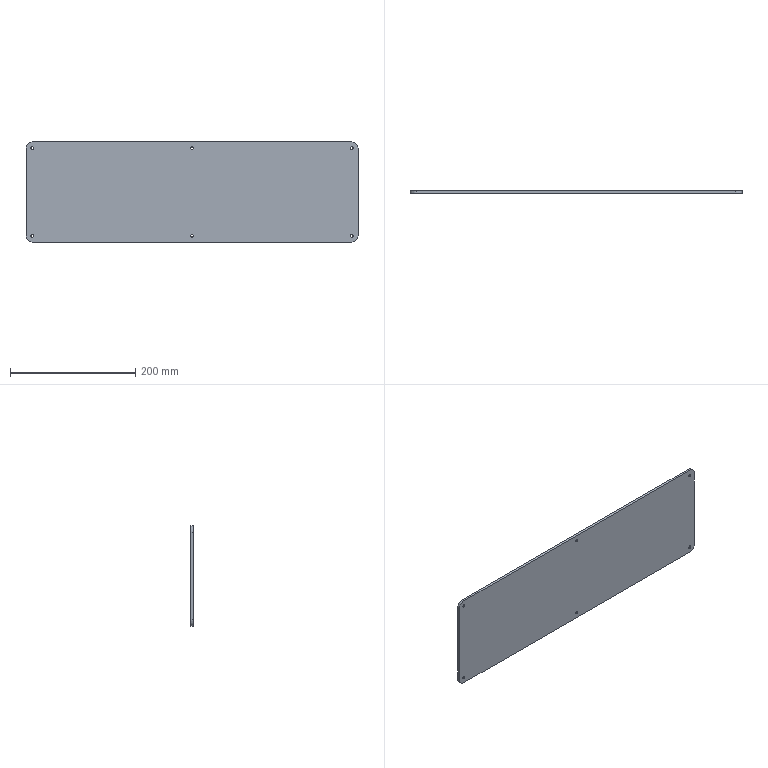Part | NX | 1 solid | 22 faces | box 530 x 4 x 160 mm | volume 338194 mm3 | cylinder 10 | plane 6 | cone 6 | commonest cylinder face diameters 4.5 x6 20 x4
STEP:
#1=CARTESIAN_POINT('',(265.,4.,70.));
#2=VERTEX_POINT('',#1);
#3=CARTESIAN_POINT('',(265.,4.,-70.));
#4=VERTEX_POINT('',#3);
#5=CARTESIAN_POINT('',(265.,4.,-80.));
#6=DIRECTION('',(0.,0.,-1.));
#7=VECTOR('',#6,1000.);
#8=LINE('',#5,#7);
#9=EDGE_CURVE('',#2,#4,#8,.T.);
#10=ORIENTED_EDGE('',*,*,#9,.F.);
#11=CARTESIAN_POINT('',(265.,0.,70.));
#12=VERTEX_POINT('',#11);
#13=CARTESIAN_POINT('',(265.,4.,70.));
#14=DIRECTION('',(0.,-1.,0.));
#15=VECTOR('',#14,1000.);
#16=LINE('',#13,#15);
#17=EDGE_CURVE('',#2,#12,#16,.T.);
#18=ORIENTED_EDGE('',*,*,#17,.T.);
#19=CARTESIAN_POINT('',(265.,0.,-70.));
#20=VERTEX_POINT('',#19);
#21=CARTESIAN_POINT('',(265.,0.,-80.));
#22=DIRECTION('',(0.,0.,-1.));
#23=VECTOR('',#22,1000.);
#24=LINE('',#21,#23);
#25=EDGE_CURVE('',#12,#20,#24,.T.);
#26=ORIENTED_EDGE('',*,*,#25,.T.);
#27=CARTESIAN_POINT('',(265.,4.,-70.));
#28=DIRECTION('',(0.,-1.,0.));
#29=VECTOR('',#28,1000.);
#30=LINE('',#27,#29);
#31=EDGE_CURVE('',#20,#4,#30,.F.);
#32=ORIENTED_EDGE('',*,*,#31,.T.);
#33=EDGE_LOOP('',(#10,#18,#26,#32));
#34=FACE_BOUND('',#33,.T.);
#35=CARTESIAN_POINT('',(265.,4.,-80.));
#36=DIRECTION('',(-1.,0.,0.));
#37=DIRECTION('',(0.,0.,1.));
#38=AXIS2_PLACEMENT_3D('',#35,#36,#37);
#39=PLANE('',#38);
#40=ADVANCED_FACE('',(#34),#39,.F.);
#41=CARTESIAN_POINT('',(255.,4.,-80.));
#42=VERTEX_POINT('',#41);
#43=CARTESIAN_POINT('',(-255.,4.,-80.));
#44=VERTEX_POINT('',#43);
#45=CARTESIAN_POINT('',(-265.,4.,-80.));
#46=DIRECTION('',(-1.,0.,0.));
#47=VECTOR('',#46,1000.);
#48=LINE('',#45,#47);
#49=EDGE_CURVE('',#42,#44,#48,.T.);
#50=ORIENTED_EDGE('',*,*,#49,.F.);
#51=CARTESIAN_POINT('',(255.,0.,-80.));
#52=VERTEX_POINT('',#51);
#53=CARTESIAN_POINT('',(255.,4.,-80.));
#54=DIRECTION('',(0.,-1.,0.));
#55=VECTOR('',#54,1000.);
#56=LINE('',#53,#55);
#57=EDGE_CURVE('',#42,#52,#56,.T.);
#58=ORIENTED_EDGE('',*,*,#57,.T.);
#59=CARTESIAN_POINT('',(-255.,0.,-80.));
#60=VERTEX_POINT('',#59);
#61=CARTESIAN_POINT('',(-265.,0.,-80.));
#62=DIRECTION('',(-1.,0.,0.));
#63=VECTOR('',#62,1000.);
#64=LINE('',#61,#63);
#65=EDGE_CURVE('',#52,#60,#64,.T.);
#66=ORIENTED_EDGE('',*,*,#65,.T.);
#67=CARTESIAN_POINT('',(-255.,4.,-80.));
#68=DIRECTION('',(0.,-1.,0.));
#69=VECTOR('',#68,1000.);
#70=LINE('',#67,#69);
#71=EDGE_CURVE('',#60,#44,#70,.F.);
#72=ORIENTED_EDGE('',*,*,#71,.T.);
#73=EDGE_LOOP('',(#50,#58,#66,#72));
#74=FACE_BOUND('',#73,.T.);
#75=CARTESIAN_POINT('',(-265.,4.,-80.));
#76=DIRECTION('',(0.,0.,1.));
#77=DIRECTION('',(1.,0.,0.));
#78=AXIS2_PLACEMENT_3D('',#75,#76,#77);
#79=PLANE('',#78);
#80=ADVANCED_FACE('',(#74),#79,.F.);
#81=CARTESIAN_POINT('',(-265.,0.,-70.));
#82=VERTEX_POINT('',#81);
#83=CARTESIAN_POINT('',(-265.,0.,70.));
#84=VERTEX_POINT('',#83);
#85=CARTESIAN_POINT('',(-265.,0.,-80.));
#86=DIRECTION('',(0.,0.,1.));
#87=VECTOR('',#86,1000.);
#88=LINE('',#85,#87);
#89=EDGE_CURVE('',#82,#84,#88,.T.);
#90=ORIENTED_EDGE('',*,*,#89,.T.);
#91=CARTESIAN_POINT('',(-265.,4.,70.));
#92=VERTEX_POINT('',#91);
#93=CARTESIAN_POINT('',(-265.,4.,70.));
#94=DIRECTION('',(0.,-1.,0.));
#95=VECTOR('',#94,1000.);
#96=LINE('',#93,#95);
#97=EDGE_CURVE('',#84,#92,#96,.F.);
#98=ORIENTED_EDGE('',*,*,#97,.T.);
#99=CARTESIAN_POINT('',(-265.,4.,-70.));
#100=VERTEX_POINT('',#99);
#101=CARTESIAN_POINT('',(-265.,4.,-80.));
#102=DIRECTION('',(0.,0.,1.));
#103=VECTOR('',#102,1000.);
#104=LINE('',#101,#103);
#105=EDGE_CURVE('',#100,#92,#104,.T.);
#106=ORIENTED_EDGE('',*,*,#105,.F.);
#107=CARTESIAN_POINT('',(-265.,4.,-70.));
#108=DIRECTION('',(0.,-1.,0.));
#109=VECTOR('',#108,1000.);
#110=LINE('',#107,#109);
#111=EDGE_CURVE('',#100,#82,#110,.T.);
#112=ORIENTED_EDGE('',*,*,#111,.T.);
#113=EDGE_LOOP('',(#90,#98,#106,#112));
#114=FACE_BOUND('',#113,.T.);
#115=CARTESIAN_POINT('',(-265.,4.,-80.));
#116=DIRECTION('',(1.,0.,0.));
#117=DIRECTION('',(0.,0.,-1.));
#118=AXIS2_PLACEMENT_3D('',#115,#116,#117);
#119=PLANE('',#118);
#120=ADVANCED_FACE('',(#114),#119,.F.);
#121=CARTESIAN_POINT('',(-255.,0.,80.));
#122=VERTEX_POINT('',#121);
#123=CARTESIAN_POINT('',(255.,0.,80.));
#124=VERTEX_POINT('',#123);
#125=CARTESIAN_POINT('',(-265.,0.,80.));
#126=DIRECTION('',(1.,0.,0.));
#127=VECTOR('',#126,1000.);
#128=LINE('',#125,#127);
#129=EDGE_CURVE('',#122,#124,#128,.T.);
#130=ORIENTED_EDGE('',*,*,#129,.T.);
#131=CARTESIAN_POINT('',(255.,4.,80.));
#132=VERTEX_POINT('',#131);
#133=CARTESIAN_POINT('',(255.,4.,80.));
#134=DIRECTION('',(0.,-1.,0.));
#135=VECTOR('',#134,1000.);
#136=LINE('',#133,#135);
#137=EDGE_CURVE('',#124,#132,#136,.F.);
#138=ORIENTED_EDGE('',*,*,#137,.T.);
#139=CARTESIAN_POINT('',(-255.,4.,80.));
#140=VERTEX_POINT('',#139);
#141=CARTESIAN_POINT('',(-265.,4.,80.));
#142=DIRECTION('',(1.,0.,0.));
#143=VECTOR('',#142,1000.);
#144=LINE('',#141,#143);
#145=EDGE_CURVE('',#140,#132,#144,.T.);
#146=ORIENTED_EDGE('',*,*,#145,.F.);
#147=CARTESIAN_POINT('',(-255.,4.,80.));
#148=DIRECTION('',(0.,-1.,0.));
#149=VECTOR('',#148,1000.);
#150=LINE('',#147,#149);
#151=EDGE_CURVE('',#140,#122,#150,.T.);
#152=ORIENTED_EDGE('',*,*,#151,.T.);
#153=EDGE_LOOP('',(#130,#138,#146,#152));
#154=FACE_BOUND('',#153,.T.);
#155=CARTESIAN_POINT('',(-265.,4.,80.));
#156=DIRECTION('',(0.,0.,-1.));
#157=DIRECTION('',(-1.,0.,0.));
#158=AXIS2_PLACEMENT_3D('',#155,#156,#157);
#159=PLANE('',#158);
#160=ADVANCED_FACE('',(#154),#159,.F.);
#161=CARTESIAN_POINT('',(-255.,4.,74.48));
#162=VERTEX_POINT('',#161);
#163=CARTESIAN_POINT('',(-255.,4.,70.));
#164=DIRECTION('',(0.,1.,0.));
#165=DIRECTION('',(0.,0.,1.));
#166=AXIS2_PLACEMENT_3D('',#163,#164,#165);
#167=CIRCLE('',#166,4.48);
#168=EDGE_CURVE('',#162,#162,#167,.T.);
#169=ORIENTED_EDGE('',*,*,#168,.F.);
#170=EDGE_LOOP('',(#169));
#171=FACE_BOUND('',#170,.T.);
#172=CARTESIAN_POINT('',(-255.,4.,-65.52));
#173=VERTEX_POINT('',#172);
#174=CARTESIAN_POINT('',(-255.,4.,-70.));
#175=DIRECTION('',(0.,1.,0.));
#176=DIRECTION('',(0.,0.,1.));
#177=AXIS2_PLACEMENT_3D('',#174,#175,#176);
#178=CIRCLE('',#177,4.48);
#179=EDGE_CURVE('',#173,#173,#178,.T.);
#180=ORIENTED_EDGE('',*,*,#179,.F.);
#181=EDGE_LOOP('',(#180));
#182=FACE_BOUND('',#181,.T.);
#183=CARTESIAN_POINT('',(255.,4.,74.48));
#184=VERTEX_POINT('',#183);
#185=CARTESIAN_POINT('',(255.,4.,70.));
#186=DIRECTION('',(0.,1.,0.));
#187=DIRECTION('',(0.,0.,1.));
#188=AXIS2_PLACEMENT_3D('',#185,#186,#187);
#189=CIRCLE('',#188,4.48);
#190=EDGE_CURVE('',#184,#184,#189,.T.);
#191=ORIENTED_EDGE('',*,*,#190,.F.);
#192=EDGE_LOOP('',(#191));
#193=FACE_BOUND('',#192,.T.);
#194=CARTESIAN_POINT('',(255.,4.,-65.52));
#195=VERTEX_POINT('',#194);
#196=CARTESIAN_POINT('',(255.,4.,-70.));
#197=DIRECTION('',(0.,1.,0.));
#198=DIRECTION('',(0.,0.,1.));
#199=AXIS2_PLACEMENT_3D('',#196,#197,#198);
#200=CIRCLE('',#199,4.48);
#201=EDGE_CURVE('',#195,#195,#200,.T.);
#202=ORIENTED_EDGE('',*,*,#201,.F.);
#203=EDGE_LOOP('',(#202));
#204=FACE_BOUND('',#203,.T.);
#205=CARTESIAN_POINT('',(0.,4.,-65.52));
#206=VERTEX_POINT('',#205);
#207=CARTESIAN_POINT('',(0.,4.,-70.));
#208=DIRECTION('',(0.,1.,0.));
#209=DIRECTION('',(0.,0.,1.));
#210=AXIS2_PLACEMENT_3D('',#207,#208,#209);
#211=CIRCLE('',#210,4.48);
#212=EDGE_CURVE('',#206,#206,#211,.T.);
#213=ORIENTED_EDGE('',*,*,#212,.F.);
#214=EDGE_LOOP('',(#213));
#215=FACE_BOUND('',#214,.T.);
#216=CARTESIAN_POINT('',(0.,4.,74.48));
#217=VERTEX_POINT('',#216);
#218=CARTESIAN_POINT('',(0.,4.,70.));
#219=DIRECTION('',(0.,1.,0.));
#220=DIRECTION('',(0.,0.,1.));
#221=AXIS2_PLACEMENT_3D('',#218,#219,#220);
#222=CIRCLE('',#221,4.48);
#223=EDGE_CURVE('',#217,#217,#222,.T.);
#224=ORIENTED_EDGE('',*,*,#223,.F.);
#225=EDGE_LOOP('',(#224));
#226=FACE_BOUND('',#225,.T.);
#227=ORIENTED_EDGE('',*,*,#145,.T.);
#228=CARTESIAN_POINT('',(255.,4.,70.));
#229=DIRECTION('',(0.,1.,0.));
#230=DIRECTION('',(0.,0.,1.));
#231=AXIS2_PLACEMENT_3D('',#228,#229,#230);
#232=CIRCLE('',#231,10.);
#233=EDGE_CURVE('',#132,#2,#232,.T.);
#234=ORIENTED_EDGE('',*,*,#233,.T.);
#235=ORIENTED_EDGE('',*,*,#9,.T.);
#236=CARTESIAN_POINT('',(255.,4.,-70.));
#237=DIRECTION('',(0.,1.,0.));
#238=DIRECTION('',(0.,0.,1.));
#239=AXIS2_PLACEMENT_3D('',#236,#237,#238);
#240=CIRCLE('',#239,10.);
#241=EDGE_CURVE('',#4,#42,#240,.T.);
#242=ORIENTED_EDGE('',*,*,#241,.T.);
#243=ORIENTED_EDGE('',*,*,#49,.T.);
#244=CARTESIAN_POINT('',(-255.,4.,-70.));
#245=DIRECTION('',(0.,1.,0.));
#246=DIRECTION('',(0.,0.,1.));
#247=AXIS2_PLACEMENT_3D('',#244,#245,#246);
#248=CIRCLE('',#247,10.);
#249=EDGE_CURVE('',#44,#100,#248,.T.);
#250=ORIENTED_EDGE('',*,*,#249,.T.);
#251=ORIENTED_EDGE('',*,*,#105,.T.);
#252=CARTESIAN_POINT('',(-255.,4.,70.));
#253=DIRECTION('',(0.,1.,0.));
#254=DIRECTION('',(0.,0.,1.));
#255=AXIS2_PLACEMENT_3D('',#252,#253,#254);
#256=CIRCLE('',#255,10.);
#257=EDGE_CURVE('',#92,#140,#256,.T.);
#258=ORIENTED_EDGE('',*,*,#257,.T.);
#259=EDGE_LOOP('',(#227,#234,#235,#242,#243,#250,#251,#258));
#260=FACE_BOUND('',#259,.T.);
#261=CARTESIAN_POINT('',(0.,4.,0.));
#262=DIRECTION('',(0.,1.,0.));
#263=DIRECTION('',(0.,0.,1.));
#264=AXIS2_PLACEMENT_3D('',#261,#262,#263);
#265=PLANE('',#264);
#266=ADVANCED_FACE('',(#171,#182,#193,#204,#215,#226,#260),#265,.T.);
#267=CARTESIAN_POINT('',(-255.,0.,72.25));
#268=VERTEX_POINT('',#267);
#269=CARTESIAN_POINT('',(-255.,0.,70.));
#270=DIRECTION('',(0.,1.,0.));
#271=DIRECTION('',(0.,0.,1.));
#272=AXIS2_PLACEMENT_3D('',#269,#270,#271);
#273=CIRCLE('',#272,2.25);
#274=EDGE_CURVE('',#268,#268,#273,.T.);
#275=ORIENTED_EDGE('',*,*,#274,.T.);
#276=EDGE_LOOP('',(#275));
#277=FACE_BOUND('',#276,.T.);
#278=CARTESIAN_POINT('',(-255.,0.,-67.75));
#279=VERTEX_POINT('',#278);
#280=CARTESIAN_POINT('',(-255.,0.,-70.));
#281=DIRECTION('',(0.,1.,0.));
#282=DIRECTION('',(0.,0.,1.));
#283=AXIS2_PLACEMENT_3D('',#280,#281,#282);
#284=CIRCLE('',#283,2.25);
#285=EDGE_CURVE('',#279,#279,#284,.T.);
#286=ORIENTED_EDGE('',*,*,#285,.T.);
#287=EDGE_LOOP('',(#286));
#288=FACE_BOUND('',#287,.T.);
#289=CARTESIAN_POINT('',(255.,0.,72.25));
#290=VERTEX_POINT('',#289);
#291=CARTESIAN_POINT('',(255.,0.,70.));
#292=DIRECTION('',(0.,1.,0.));
#293=DIRECTION('',(0.,0.,1.));
#294=AXIS2_PLACEMENT_3D('',#291,#292,#293);
#295=CIRCLE('',#294,2.25);
#296=EDGE_CURVE('',#290,#290,#295,.T.);
#297=ORIENTED_EDGE('',*,*,#296,.T.);
#298=EDGE_LOOP('',(#297));
#299=FACE_BOUND('',#298,.T.);
#300=CARTESIAN_POINT('',(255.,0.,-67.75));
#301=VERTEX_POINT('',#300);
#302=CARTESIAN_POINT('',(255.,0.,-70.));
#303=DIRECTION('',(0.,1.,0.));
#304=DIRECTION('',(0.,0.,1.));
#305=AXIS2_PLACEMENT_3D('',#302,#303,#304);
#306=CIRCLE('',#305,2.25);
#307=EDGE_CURVE('',#301,#301,#306,.T.);
#308=ORIENTED_EDGE('',*,*,#307,.T.);
#309=EDGE_LOOP('',(#308));
#310=FACE_BOUND('',#309,.T.);
#311=CARTESIAN_POINT('',(0.,0.,-67.75));
#312=VERTEX_POINT('',#311);
#313=CARTESIAN_POINT('',(0.,0.,-70.));
#314=DIRECTION('',(0.,1.,0.));
#315=DIRECTION('',(0.,0.,1.));
#316=AXIS2_PLACEMENT_3D('',#313,#314,#315);
#317=CIRCLE('',#316,2.25);
#318=EDGE_CURVE('',#312,#312,#317,.T.);
#319=ORIENTED_EDGE('',*,*,#318,.T.);
#320=EDGE_LOOP('',(#319));
#321=FACE_BOUND('',#320,.T.);
#322=CARTESIAN_POINT('',(0.,0.,72.25));
#323=VERTEX_POINT('',#322);
#324=CARTESIAN_POINT('',(0.,0.,70.));
#325=DIRECTION('',(0.,1.,0.));
#326=DIRECTION('',(0.,0.,1.));
#327=AXIS2_PLACEMENT_3D('',#324,#325,#326);
#328=CIRCLE('',#327,2.25);
#329=EDGE_CURVE('',#323,#323,#328,.T.);
#330=ORIENTED_EDGE('',*,*,#329,.T.);
#331=EDGE_LOOP('',(#330));
#332=FACE_BOUND('',#331,.T.);
#333=ORIENTED_EDGE('',*,*,#25,.F.);
#334=CARTESIAN_POINT('',(255.,0.,70.));
#335=DIRECTION('',(0.,1.,0.));
#336=DIRECTION('',(0.,0.,1.));
#337=AXIS2_PLACEMENT_3D('',#334,#335,#336);
#338=CIRCLE('',#337,10.);
#339=EDGE_CURVE('',#12,#124,#338,.F.);
#340=ORIENTED_EDGE('',*,*,#339,.T.);
#341=ORIENTED_EDGE('',*,*,#129,.F.);
#342=CARTESIAN_POINT('',(-255.,0.,70.));
#343=DIRECTION('',(0.,1.,0.));
#344=DIRECTION('',(0.,0.,1.));
#345=AXIS2_PLACEMENT_3D('',#342,#343,#344);
#346=CIRCLE('',#345,10.);
#347=EDGE_CURVE('',#122,#84,#346,.F.);
#348=ORIENTED_EDGE('',*,*,#347,.T.);
#349=ORIENTED_EDGE('',*,*,#89,.F.);
#350=CARTESIAN_POINT('',(-255.,0.,-70.));
#351=DIRECTION('',(0.,1.,0.));
#352=DIRECTION('',(0.,0.,1.));
#353=AXIS2_PLACEMENT_3D('',#350,#351,#352);
#354=CIRCLE('',#353,10.);
#355=EDGE_CURVE('',#82,#60,#354,.F.);
#356=ORIENTED_EDGE('',*,*,#355,.T.);
#357=ORIENTED_EDGE('',*,*,#65,.F.);
#358=CARTESIAN_POINT('',(255.,0.,-70.));
#359=DIRECTION('',(0.,1.,0.));
#360=DIRECTION('',(0.,0.,1.));
#361=AXIS2_PLACEMENT_3D('',#358,#359,#360);
#362=CIRCLE('',#361,10.);
#363=EDGE_CURVE('',#52,#20,#362,.F.);
#364=ORIENTED_EDGE('',*,*,#363,.T.);
#365=EDGE_LOOP('',(#333,#340,#341,#348,#349,#356,#357,#364));
#366=FACE_BOUND('',#365,.T.);
#367=CARTESIAN_POINT('',(0.,0.,0.));
#368=DIRECTION('',(0.,1.,0.));
#369=DIRECTION('',(0.,0.,1.));
#370=AXIS2_PLACEMENT_3D('',#367,#368,#369);
#371=PLANE('',#370);
#372=ADVANCED_FACE('',(#277,#288,#299,#310,#321,#332,#366),#371,.F.);
#373=ORIENTED_EDGE('',*,*,#329,.F.);
#374=EDGE_LOOP('',(#373));
#375=FACE_BOUND('',#374,.T.);
#376=CARTESIAN_POINT('',(0.,1.77,72.25));
#377=VERTEX_POINT('',#376);
#378=CARTESIAN_POINT('',(0.,1.77,70.));
#379=DIRECTION('',(0.,1.,0.));
#380=DIRECTION('',(0.,0.,1.));
#381=AXIS2_PLACEMENT_3D('',#378,#379,#380);
#382=CIRCLE('',#381,2.25);
#383=EDGE_CURVE('',#377,#377,#382,.T.);
#384=ORIENTED_EDGE('',*,*,#383,.T.);
#385=EDGE_LOOP('',(#384));
#386=FACE_BOUND('',#385,.T.);
#387=CARTESIAN_POINT('',(0.,4.,70.));
#388=DIRECTION('',(0.,1.,0.));
#389=DIRECTION('',(0.,0.,1.));
#390=AXIS2_PLACEMENT_3D('',#387,#388,#389);
#391=CYLINDRICAL_SURFACE('',#390,2.25);
#392=ADVANCED_FACE('',(#375,#386),#391,.F.);
#393=ORIENTED_EDGE('',*,*,#383,.F.);
#394=EDGE_LOOP('',(#393));
#395=FACE_BOUND('',#394,.T.);
#396=ORIENTED_EDGE('',*,*,#223,.T.);
#397=EDGE_LOOP('',(#396));
#398=FACE_BOUND('',#397,.T.);
#399=CARTESIAN_POINT('',(0.,4.,70.));
#400=DIRECTION('',(0.,1.,0.));
#401=DIRECTION('',(0.,0.,1.));
#402=AXIS2_PLACEMENT_3D('',#399,#400,#401);
#403=CONICAL_SURFACE('',#402,4.48,0.7854);
#404=ADVANCED_FACE('',(#395,#398),#403,.F.);
#405=ORIENTED_EDGE('',*,*,#318,.F.);
#406=EDGE_LOOP('',(#405));
#407=FACE_BOUND('',#406,.T.);
#408=CARTESIAN_POINT('',(0.,1.77,-67.75));
#409=VERTEX_POINT('',#408);
#410=CARTESIAN_POINT('',(0.,1.77,-70.));
#411=DIRECTION('',(0.,1.,0.));
#412=DIRECTION('',(0.,0.,1.));
#413=AXIS2_PLACEMENT_3D('',#410,#411,#412);
#414=CIRCLE('',#413,2.25);
#415=EDGE_CURVE('',#409,#409,#414,.T.);
#416=ORIENTED_EDGE('',*,*,#415,.T.);
#417=EDGE_LOOP('',(#416));
#418=FACE_BOUND('',#417,.T.);
#419=CARTESIAN_POINT('',(0.,4.,-70.));
#420=DIRECTION('',(0.,1.,0.));
#421=DIRECTION('',(0.,0.,1.));
#422=AXIS2_PLACEMENT_3D('',#419,#420,#421);
#423=CYLINDRICAL_SURFACE('',#422,2.25);
#424=ADVANCED_FACE('',(#407,#418),#423,.F.);
#425=ORIENTED_EDGE('',*,*,#415,.F.);
#426=EDGE_LOOP('',(#425));
#427=FACE_BOUND('',#426,.T.);
#428=ORIENTED_EDGE('',*,*,#212,.T.);
#429=EDGE_LOOP('',(#428));
#430=FACE_BOUND('',#429,.T.);
#431=CARTESIAN_POINT('',(0.,4.,-70.));
#432=DIRECTION('',(0.,1.,0.));
#433=DIRECTION('',(0.,0.,1.));
#434=AXIS2_PLACEMENT_3D('',#431,#432,#433);
#435=CONICAL_SURFACE('',#434,4.48,0.7854);
#436=ADVANCED_FACE('',(#427,#430),#435,.F.);
#437=ORIENTED_EDGE('',*,*,#307,.F.);
#438=EDGE_LOOP('',(#437));
#439=FACE_BOUND('',#438,.T.);
#440=CARTESIAN_POINT('',(255.,1.77,-67.75));
#441=VERTEX_POINT('',#440);
#442=CARTESIAN_POINT('',(255.,1.77,-70.));
#443=DIRECTION('',(0.,1.,0.));
#444=DIRECTION('',(0.,0.,1.));
#445=AXIS2_PLACEMENT_3D('',#442,#443,#444);
#446=CIRCLE('',#445,2.25);
#447=EDGE_CURVE('',#441,#441,#446,.T.);
#448=ORIENTED_EDGE('',*,*,#447,.T.);
#449=EDGE_LOOP('',(#448));
#450=FACE_BOUND('',#449,.T.);
#451=CARTESIAN_POINT('',(255.,4.,-70.));
#452=DIRECTION('',(0.,1.,0.));
#453=DIRECTION('',(0.,0.,1.));
#454=AXIS2_PLACEMENT_3D('',#451,#452,#453);
#455=CYLINDRICAL_SURFACE('',#454,2.25);
#456=ADVANCED_FACE('',(#439,#450),#455,.F.);
#457=ORIENTED_EDGE('',*,*,#447,.F.);
#458=EDGE_LOOP('',(#457));
#459=FACE_BOUND('',#458,.T.);
#460=ORIENTED_EDGE('',*,*,#201,.T.);
#461=EDGE_LOOP('',(#460));
#462=FACE_BOUND('',#461,.T.);
#463=CARTESIAN_POINT('',(255.,4.,-70.));
#464=DIRECTION('',(0.,1.,0.));
#465=DIRECTION('',(0.,0.,1.));
#466=AXIS2_PLACEMENT_3D('',#463,#464,#465);
#467=CONICAL_SURFACE('',#466,4.48,0.7854);
#468=ADVANCED_FACE('',(#459,#462),#467,.F.);
#469=ORIENTED_EDGE('',*,*,#296,.F.);
#470=EDGE_LOOP('',(#469));
#471=FACE_BOUND('',#470,.T.);
#472=CARTESIAN_POINT('',(255.,1.77,72.25));
#473=VERTEX_POINT('',#472);
#474=CARTESIAN_POINT('',(255.,1.77,70.));
#475=DIRECTION('',(0.,1.,0.));
#476=DIRECTION('',(0.,0.,1.));
#477=AXIS2_PLACEMENT_3D('',#474,#475,#476);
#478=CIRCLE('',#477,2.25);
#479=EDGE_CURVE('',#473,#473,#478,.T.);
#480=ORIENTED_EDGE('',*,*,#479,.T.);
#481=EDGE_LOOP('',(#480));
#482=FACE_BOUND('',#481,.T.);
#483=CARTESIAN_POINT('',(255.,4.,70.));
#484=DIRECTION('',(0.,1.,0.));
#485=DIRECTION('',(0.,0.,1.));
#486=AXIS2_PLACEMENT_3D('',#483,#484,#485);
#487=CYLINDRICAL_SURFACE('',#486,2.25);
#488=ADVANCED_FACE('',(#471,#482),#487,.F.);
#489=ORIENTED_EDGE('',*,*,#479,.F.);
#490=EDGE_LOOP('',(#489));
#491=FACE_BOUND('',#490,.T.);
#492=ORIENTED_EDGE('',*,*,#190,.T.);
#493=EDGE_LOOP('',(#492));
#494=FACE_BOUND('',#493,.T.);
#495=CARTESIAN_POINT('',(255.,4.,70.));
#496=DIRECTION('',(0.,1.,0.));
#497=DIRECTION('',(0.,0.,1.));
#498=AXIS2_PLACEMENT_3D('',#495,#496,#497);
#499=CONICAL_SURFACE('',#498,4.48,0.7854);
#500=ADVANCED_FACE('',(#491,#494),#499,.F.);
#501=ORIENTED_EDGE('',*,*,#285,.F.);
#502=EDGE_LOOP('',(#501));
#503=FACE_BOUND('',#502,.T.);
#504=CARTESIAN_POINT('',(-255.,1.77,-67.75));
#505=VERTEX_POINT('',#504);
#506=CARTESIAN_POINT('',(-255.,1.77,-70.));
#507=DIRECTION('',(0.,1.,0.));
#508=DIRECTION('',(0.,0.,1.));
#509=AXIS2_PLACEMENT_3D('',#506,#507,#508);
#510=CIRCLE('',#509,2.25);
#511=EDGE_CURVE('',#505,#505,#510,.T.);
#512=ORIENTED_EDGE('',*,*,#511,.T.);
#513=EDGE_LOOP('',(#512));
#514=FACE_BOUND('',#513,.T.);
#515=CARTESIAN_POINT('',(-255.,4.,-70.));
#516=DIRECTION('',(0.,1.,0.));
#517=DIRECTION('',(0.,0.,1.));
#518=AXIS2_PLACEMENT_3D('',#515,#516,#517);
#519=CYLINDRICAL_SURFACE('',#518,2.25);
#520=ADVANCED_FACE('',(#503,#514),#519,.F.);
#521=ORIENTED_EDGE('',*,*,#511,.F.);
#522=EDGE_LOOP('',(#521));
#523=FACE_BOUND('',#522,.T.);
#524=ORIENTED_EDGE('',*,*,#179,.T.);
#525=EDGE_LOOP('',(#524));
#526=FACE_BOUND('',#525,.T.);
#527=CARTESIAN_POINT('',(-255.,4.,-70.));
#528=DIRECTION('',(0.,1.,0.));
#529=DIRECTION('',(0.,0.,1.));
#530=AXIS2_PLACEMENT_3D('',#527,#528,#529);
#531=CONICAL_SURFACE('',#530,4.48,0.7854);
#532=ADVANCED_FACE('',(#523,#526),#531,.F.);
#533=ORIENTED_EDGE('',*,*,#274,.F.);
#534=EDGE_LOOP('',(#533));
#535=FACE_BOUND('',#534,.T.);
#536=CARTESIAN_POINT('',(-255.,1.77,72.25));
#537=VERTEX_POINT('',#536);
#538=CARTESIAN_POINT('',(-255.,1.77,70.));
#539=DIRECTION('',(0.,1.,0.));
#540=DIRECTION('',(0.,0.,1.));
#541=AXIS2_PLACEMENT_3D('',#538,#539,#540);
#542=CIRCLE('',#541,2.25);
#543=EDGE_CURVE('',#537,#537,#542,.T.);
#544=ORIENTED_EDGE('',*,*,#543,.T.);
#545=EDGE_LOOP('',(#544));
#546=FACE_BOUND('',#545,.T.);
#547=CARTESIAN_POINT('',(-255.,4.,70.));
#548=DIRECTION('',(0.,1.,0.));
#549=DIRECTION('',(0.,0.,1.));
#550=AXIS2_PLACEMENT_3D('',#547,#548,#549);
#551=CYLINDRICAL_SURFACE('',#550,2.25);
#552=ADVANCED_FACE('',(#535,#546),#551,.F.);
#553=ORIENTED_EDGE('',*,*,#543,.F.);
#554=EDGE_LOOP('',(#553));
#555=FACE_BOUND('',#554,.T.);
#556=ORIENTED_EDGE('',*,*,#168,.T.);
#557=EDGE_LOOP('',(#556));
#558=FACE_BOUND('',#557,.T.);
#559=CARTESIAN_POINT('',(-255.,4.,70.));
#560=DIRECTION('',(0.,1.,0.));
#561=DIRECTION('',(0.,0.,1.));
#562=AXIS2_PLACEMENT_3D('',#559,#560,#561);
#563=CONICAL_SURFACE('',#562,4.48,0.7854);
#564=ADVANCED_FACE('',(#555,#558),#563,.F.);
#565=ORIENTED_EDGE('',*,*,#233,.F.);
#566=ORIENTED_EDGE('',*,*,#137,.F.);
#567=ORIENTED_EDGE('',*,*,#339,.F.);
#568=ORIENTED_EDGE('',*,*,#17,.F.);
#569=EDGE_LOOP('',(#565,#566,#567,#568));
#570=FACE_BOUND('',#569,.T.);
#571=CARTESIAN_POINT('',(255.,4.,70.));
#572=DIRECTION('',(0.,-1.,0.));
#573=DIRECTION('',(0.,0.,-1.));
#574=AXIS2_PLACEMENT_3D('',#571,#572,#573);
#575=CYLINDRICAL_SURFACE('',#574,10.);
#576=ADVANCED_FACE('',(#570),#575,.T.);
#577=ORIENTED_EDGE('',*,*,#241,.F.);
#578=ORIENTED_EDGE('',*,*,#31,.F.);
#579=ORIENTED_EDGE('',*,*,#363,.F.);
#580=ORIENTED_EDGE('',*,*,#57,.F.);
#581=EDGE_LOOP('',(#577,#578,#579,#580));
#582=FACE_BOUND('',#581,.T.);
#583=CARTESIAN_POINT('',(255.,4.,-70.));
#584=DIRECTION('',(0.,-1.,0.));
#585=DIRECTION('',(0.,0.,-1.));
#586=AXIS2_PLACEMENT_3D('',#583,#584,#585);
#587=CYLINDRICAL_SURFACE('',#586,10.);
#588=ADVANCED_FACE('',(#582),#587,.T.);
#589=ORIENTED_EDGE('',*,*,#257,.F.);
#590=ORIENTED_EDGE('',*,*,#97,.F.);
#591=ORIENTED_EDGE('',*,*,#347,.F.);
#592=ORIENTED_EDGE('',*,*,#151,.F.);
#593=EDGE_LOOP('',(#589,#590,#591,#592));
#594=FACE_BOUND('',#593,.T.);
#595=CARTESIAN_POINT('',(-255.,4.,70.));
#596=DIRECTION('',(0.,-1.,0.));
#597=DIRECTION('',(0.,0.,-1.));
#598=AXIS2_PLACEMENT_3D('',#595,#596,#597);
#599=CYLINDRICAL_SURFACE('',#598,10.);
#600=ADVANCED_FACE('',(#594),#599,.T.);
#601=ORIENTED_EDGE('',*,*,#249,.F.);
#602=ORIENTED_EDGE('',*,*,#71,.F.);
#603=ORIENTED_EDGE('',*,*,#355,.F.);
#604=ORIENTED_EDGE('',*,*,#111,.F.);
#605=EDGE_LOOP('',(#601,#602,#603,#604));
#606=FACE_BOUND('',#605,.T.);
#607=CARTESIAN_POINT('',(-255.,4.,-70.));
#608=DIRECTION('',(0.,-1.,0.));
#609=DIRECTION('',(0.,0.,-1.));
#610=AXIS2_PLACEMENT_3D('',#607,#608,#609);
#611=CYLINDRICAL_SURFACE('',#610,10.);
#612=ADVANCED_FACE('',(#606),#611,.T.);
#613=CLOSED_SHELL('',(#40,#80,#120,#160,#266,#372,#392,#404,#424,#436,#456,#468,#488,#500,#520,#532,#552,#564,#576,#588,#600,#612));
#614=MANIFOLD_SOLID_BREP('',#613);
#615=(LENGTH_UNIT()NAMED_UNIT(*)SI_UNIT(.MILLI.,.METRE.));
#616=UNCERTAINTY_MEASURE_WITH_UNIT(LENGTH_MEASURE(0.00001),#615,'','');
#617=(NAMED_UNIT(*)PLANE_ANGLE_UNIT()SI_UNIT($,.RADIAN.));
#618=(NAMED_UNIT(*)SI_UNIT($,.STERADIAN.)SOLID_ANGLE_UNIT());
#619=(GEOMETRIC_REPRESENTATION_CONTEXT(3)GLOBAL_UNCERTAINTY_ASSIGNED_CONTEXT((#616))GLOBAL_UNIT_ASSIGNED_CONTEXT((#615,#617,#618))REPRESENTATION_CONTEXT('',''));
#620=ADVANCED_BREP_SHAPE_REPRESENTATION('',(#614),#619);